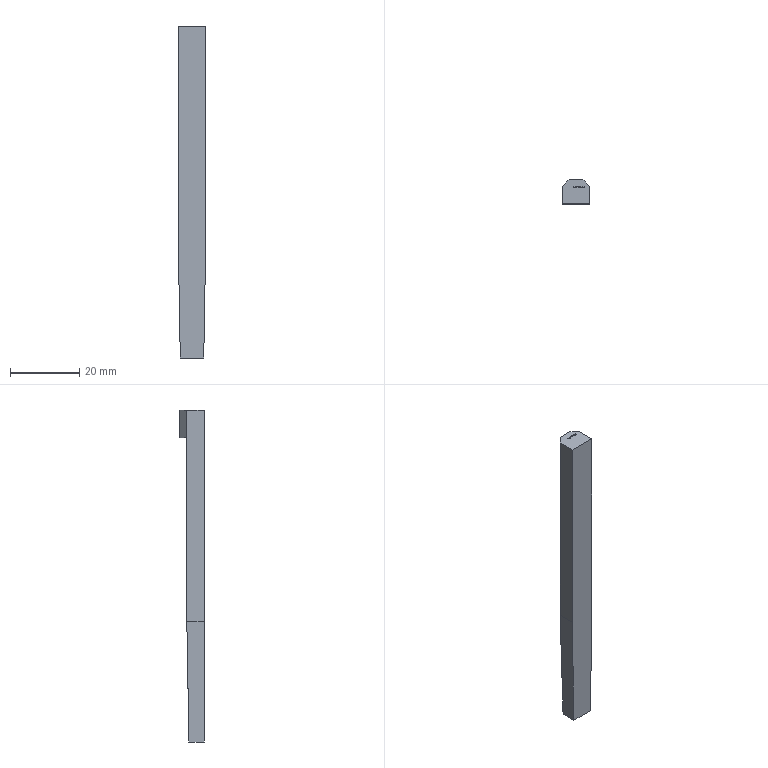Part | Creo | 1 solid | 114 faces | box 8.004 x 6.997 x 95.989 mm | volume 3752 mm3 | other 66 | plane 47 | cylinder 1 | commonest cylinder face diameters 0.39 x1